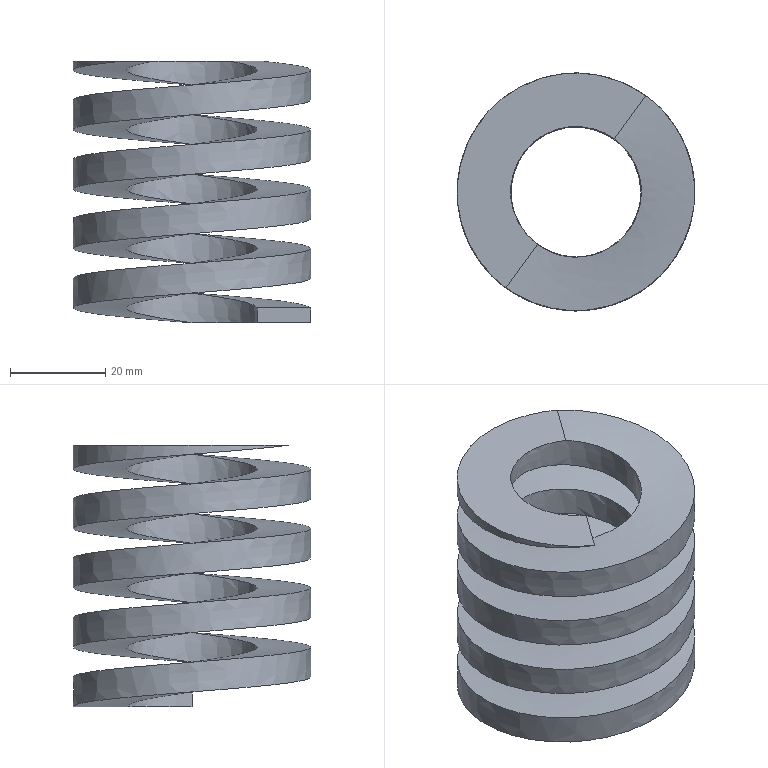Part | Creo | 1 solid | 7 faces | box 50 x 50 x 55 mm | volume 36929 mm3 | spline 4 | plane 3